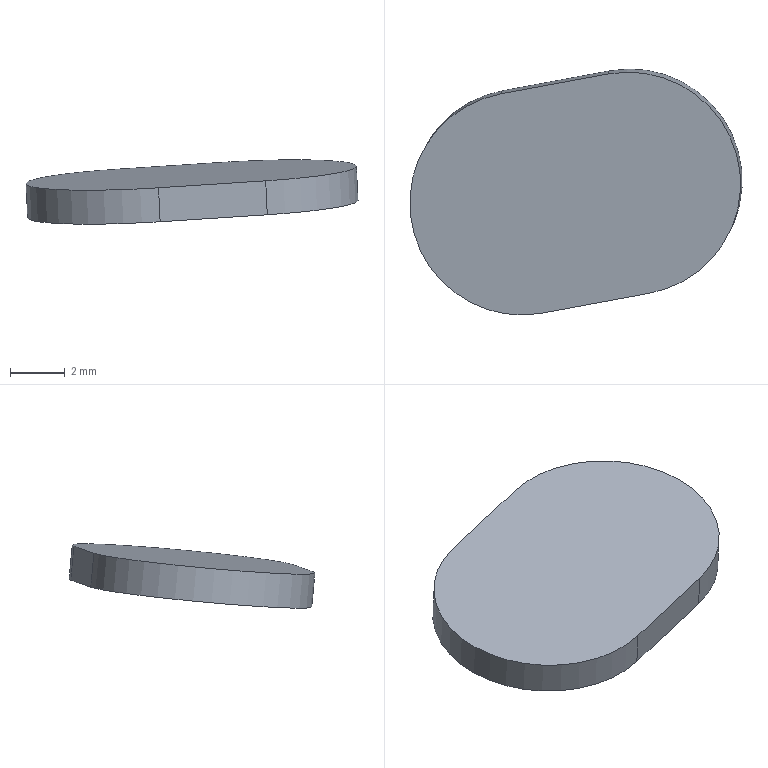Part | STEP file | gslz 2016.10.28-13_id1330_x_t | 1 solid | 6 faces | box 12.175 x 9.008 x 2.356 mm | volume 107.013 mm3 | plane 4 | cylinder 2 | commonest cylinder face diameters 8.2 x2
STEP:
#1=CARTESIAN_POINT('',(0.,0.,0.));
#2=DIRECTION('',(0.,0.,1.));
#3=DIRECTION('',(1.,0.,0.));
#4=AXIS2_PLACEMENT_3D('',#1,#2,#3);
#5=CARTESIAN_POINT('',(1413.762,14.955,-0.7524));
#6=VERTEX_POINT('',#5);
#7=CARTESIAN_POINT('',(1412.231,22.982,-0.07377));
#8=VERTEX_POINT('',#7);
#9=CARTESIAN_POINT('',(1412.996,18.968,-0.4131));
#10=DIRECTION('',(0.04745,0.09314,-0.9945));
#11=DIRECTION('',(0.4515,0.8861,0.1045));
#12=AXIS2_PLACEMENT_3D('',#9,#10,#11);
#13=CIRCLE('',#12,4.1);
#14=CARTESIAN_POINT('',(1413.056,19.085,-1.656));
#15=DIRECTION('',(-0.04745,-0.09314,0.9945));
#16=DIRECTION('',(0.,-0.9956,-0.09324));
#17=AXIS2_PLACEMENT_3D('',#14,#15,#16);
#18=CYLINDRICAL_SURFACE('',#17,4.1);
#19=CARTESIAN_POINT('',(8.956,1.25));
#20=DIRECTION('',(-1.,0.));
#21=VECTOR('',#20,1.);
#22=LINE('',#19,#21);
#23=(GEOMETRIC_REPRESENTATION_CONTEXT(2)PARAMETRIC_REPRESENTATION_CONTEXT()REPRESENTATION_CONTEXT('',''));
#24=DEFINITIONAL_REPRESENTATION('',(#22),#23);
#25=PCURVE('',#18,#24);
#26=CARTESIAN_POINT('',(1412.996,18.968,-0.4131));
#27=DIRECTION('',(0.04745,0.09314,-0.9945));
#28=DIRECTION('',(0.,0.9956,0.09324));
#29=AXIS2_PLACEMENT_3D('',#26,#27,#28);
#30=PLANE('',#29);
#31=CARTESIAN_POINT('',(0.,0.));
#32=DIRECTION('',(0.892,0.452));
#33=AXIS2_PLACEMENT_2D('',#31,#32);
#34=CIRCLE('',#33,4.1);
#35=(GEOMETRIC_REPRESENTATION_CONTEXT(2)PARAMETRIC_REPRESENTATION_CONTEXT()REPRESENTATION_CONTEXT('',''));
#36=DEFINITIONAL_REPRESENTATION('',(#34),#35);
#37=PCURVE('',#30,#36);
#38=SURFACE_CURVE('',#13,(#25,#37),.PCURVE_S1.);
#39=EDGE_CURVE('',#6,#8,#38,.T.);
#40=ORIENTED_EDGE('',*,*,#39,.T.);
#41=CARTESIAN_POINT('',(1412.29,23.098,-1.317));
#42=VERTEX_POINT('',#41);
#43=CARTESIAN_POINT('',(1412.29,23.098,-1.317));
#44=DIRECTION('',(-0.04745,-0.09314,0.9945));
#45=VECTOR('',#44,1.);
#46=LINE('',#43,#45);
#47=CARTESIAN_POINT('',(3.33,0.));
#48=DIRECTION('',(0.,1.));
#49=VECTOR('',#48,1.);
#50=LINE('',#47,#49);
#51=(GEOMETRIC_REPRESENTATION_CONTEXT(2)PARAMETRIC_REPRESENTATION_CONTEXT()REPRESENTATION_CONTEXT('',''));
#52=DEFINITIONAL_REPRESENTATION('',(#50),#51);
#53=PCURVE('',#18,#52);
#54=CARTESIAN_POINT('',(1412.29,23.098,-1.317));
#55=DIRECTION('',(0.1867,-0.9789,-0.08276));
#56=DIRECTION('',(0.9823,0.1874,0.));
#57=AXIS2_PLACEMENT_3D('',#54,#55,#56);
#58=PLANE('',#57);
#59=CARTESIAN_POINT('',(0.,0.));
#60=DIRECTION('',(-0.06407,0.9979));
#61=VECTOR('',#60,1.);
#62=LINE('',#59,#61);
#63=(GEOMETRIC_REPRESENTATION_CONTEXT(2)PARAMETRIC_REPRESENTATION_CONTEXT()REPRESENTATION_CONTEXT('',''));
#64=DEFINITIONAL_REPRESENTATION('',(#62),#63);
#65=PCURVE('',#58,#64);
#66=SURFACE_CURVE('',#46,(#53,#65),.PCURVE_S1.);
#67=EDGE_CURVE('',#42,#8,#66,.T.);
#68=ORIENTED_EDGE('',*,*,#67,.F.);
#69=CARTESIAN_POINT('',(1413.821,15.071,-1.996));
#70=VERTEX_POINT('',#69);
#71=CARTESIAN_POINT('',(1413.056,19.085,-1.656));
#72=DIRECTION('',(0.04745,0.09314,-0.9945));
#73=DIRECTION('',(0.4515,0.8861,0.1045));
#74=AXIS2_PLACEMENT_3D('',#71,#72,#73);
#75=CIRCLE('',#74,4.1);
#76=CARTESIAN_POINT('',(8.956,0.));
#77=DIRECTION('',(-1.,0.));
#78=VECTOR('',#77,1.);
#79=LINE('',#76,#78);
#80=(GEOMETRIC_REPRESENTATION_CONTEXT(2)PARAMETRIC_REPRESENTATION_CONTEXT()REPRESENTATION_CONTEXT('',''));
#81=DEFINITIONAL_REPRESENTATION('',(#79),#80);
#82=PCURVE('',#18,#81);
#83=CARTESIAN_POINT('',(1413.056,19.085,-1.656));
#84=DIRECTION('',(0.04745,0.09314,-0.9945));
#85=DIRECTION('',(0.,0.9956,0.09324));
#86=AXIS2_PLACEMENT_3D('',#83,#84,#85);
#87=PLANE('',#86);
#88=CARTESIAN_POINT('',(0.,0.));
#89=DIRECTION('',(0.892,0.452));
#90=AXIS2_PLACEMENT_2D('',#88,#89);
#91=CIRCLE('',#90,4.1);
#92=(GEOMETRIC_REPRESENTATION_CONTEXT(2)PARAMETRIC_REPRESENTATION_CONTEXT()REPRESENTATION_CONTEXT('',''));
#93=DEFINITIONAL_REPRESENTATION('',(#91),#92);
#94=PCURVE('',#87,#93);
#95=SURFACE_CURVE('',#75,(#82,#94),.PCURVE_S1.);
#96=EDGE_CURVE('',#70,#42,#95,.T.);
#97=ORIENTED_EDGE('',*,*,#96,.F.);
#98=CARTESIAN_POINT('',(1413.821,15.071,-1.996));
#99=DIRECTION('',(-0.04745,-0.09314,0.9945));
#100=VECTOR('',#99,1.);
#101=LINE('',#98,#100);
#102=CARTESIAN_POINT('',(6.471,0.));
#103=DIRECTION('',(0.,1.));
#104=VECTOR('',#103,1.);
#105=LINE('',#102,#104);
#106=(GEOMETRIC_REPRESENTATION_CONTEXT(2)PARAMETRIC_REPRESENTATION_CONTEXT()REPRESENTATION_CONTEXT('',''));
#107=DEFINITIONAL_REPRESENTATION('',(#105),#106);
#108=PCURVE('',#18,#107);
#109=CARTESIAN_POINT('',(1417.746,15.798,-1.74));
#110=DIRECTION('',(-0.1867,0.9789,0.08276));
#111=DIRECTION('',(-0.9823,-0.1874,0.));
#112=AXIS2_PLACEMENT_3D('',#109,#110,#111);
#113=PLANE('',#112);
#114=CARTESIAN_POINT('',(3.992,-0.2563));
#115=DIRECTION('',(0.06407,0.9979));
#116=VECTOR('',#115,1.);
#117=LINE('',#114,#116);
#118=(GEOMETRIC_REPRESENTATION_CONTEXT(2)PARAMETRIC_REPRESENTATION_CONTEXT()REPRESENTATION_CONTEXT('',''));
#119=DEFINITIONAL_REPRESENTATION('',(#117),#118);
#120=PCURVE('',#113,#119);
#121=SURFACE_CURVE('',#101,(#108,#120),.PCURVE_S1.);
#122=EDGE_CURVE('',#70,#6,#121,.T.);
#123=ORIENTED_EDGE('',*,*,#122,.T.);
#124=EDGE_LOOP('',(#40,#68,#97,#123));
#125=FACE_BOUND('',#124,.T.);
#126=ADVANCED_FACE('',(#125),#18,.T.);
#127=CARTESIAN_POINT('',(1416.156,23.709,0.1816));
#128=VERTEX_POINT('',#127);
#129=CARTESIAN_POINT('',(1412.231,22.982,-0.07377));
#130=DIRECTION('',(0.9813,0.1818,0.06385));
#131=VECTOR('',#130,1.);
#132=LINE('',#129,#131);
#133=CARTESIAN_POINT('',(-0.08008,1.247));
#134=DIRECTION('',(0.9979,0.06407));
#135=VECTOR('',#134,1.);
#136=LINE('',#133,#135);
#137=(GEOMETRIC_REPRESENTATION_CONTEXT(2)PARAMETRIC_REPRESENTATION_CONTEXT()REPRESENTATION_CONTEXT('',''));
#138=DEFINITIONAL_REPRESENTATION('',(#136),#137);
#139=PCURVE('',#58,#138);
#140=CARTESIAN_POINT('',(4.028,-0.7665));
#141=DIRECTION('',(0.1869,0.9824));
#142=VECTOR('',#141,1.);
#143=LINE('',#140,#142);
#144=(GEOMETRIC_REPRESENTATION_CONTEXT(2)PARAMETRIC_REPRESENTATION_CONTEXT()REPRESENTATION_CONTEXT('',''));
#145=DEFINITIONAL_REPRESENTATION('',(#143),#144);
#146=PCURVE('',#30,#145);
#147=SURFACE_CURVE('',#132,(#139,#146),.PCURVE_S1.);
#148=EDGE_CURVE('',#8,#128,#147,.T.);
#149=ORIENTED_EDGE('',*,*,#148,.T.);
#150=CARTESIAN_POINT('',(1416.215,23.826,-1.062));
#151=VERTEX_POINT('',#150);
#152=CARTESIAN_POINT('',(1416.215,23.826,-1.062));
#153=DIRECTION('',(-0.04745,-0.09314,0.9945));
#154=VECTOR('',#153,1.);
#155=LINE('',#152,#154);
#156=CARTESIAN_POINT('',(3.992,0.2563));
#157=DIRECTION('',(-0.06407,0.9979));
#158=VECTOR('',#157,1.);
#159=LINE('',#156,#158);
#160=(GEOMETRIC_REPRESENTATION_CONTEXT(2)PARAMETRIC_REPRESENTATION_CONTEXT()REPRESENTATION_CONTEXT('',''));
#161=DEFINITIONAL_REPRESENTATION('',(#159),#160);
#162=PCURVE('',#58,#161);
#163=CARTESIAN_POINT('',(1416.981,19.812,-1.401));
#164=DIRECTION('',(-0.04745,-0.09314,0.9945));
#165=DIRECTION('',(0.,-0.9956,-0.09324));
#166=AXIS2_PLACEMENT_3D('',#163,#164,#165);
#167=CYLINDRICAL_SURFACE('',#166,4.1);
#168=CARTESIAN_POINT('',(3.33,0.));
#169=DIRECTION('',(0.,1.));
#170=VECTOR('',#169,1.);
#171=LINE('',#168,#170);
#172=(GEOMETRIC_REPRESENTATION_CONTEXT(2)PARAMETRIC_REPRESENTATION_CONTEXT()REPRESENTATION_CONTEXT('',''));
#173=DEFINITIONAL_REPRESENTATION('',(#171),#172);
#174=PCURVE('',#167,#173);
#175=SURFACE_CURVE('',#155,(#162,#174),.PCURVE_S1.);
#176=EDGE_CURVE('',#151,#128,#175,.T.);
#177=ORIENTED_EDGE('',*,*,#176,.F.);
#178=CARTESIAN_POINT('',(1412.29,23.098,-1.317));
#179=DIRECTION('',(0.9813,0.1818,0.06385));
#180=VECTOR('',#179,1.);
#181=LINE('',#178,#180);
#182=CARTESIAN_POINT('',(0.,0.));
#183=DIRECTION('',(0.9979,0.06407));
#184=VECTOR('',#183,1.);
#185=LINE('',#182,#184);
#186=(GEOMETRIC_REPRESENTATION_CONTEXT(2)PARAMETRIC_REPRESENTATION_CONTEXT()REPRESENTATION_CONTEXT('',''));
#187=DEFINITIONAL_REPRESENTATION('',(#185),#186);
#188=PCURVE('',#58,#187);
#189=CARTESIAN_POINT('',(4.028,-0.7665));
#190=DIRECTION('',(0.1869,0.9824));
#191=VECTOR('',#190,1.);
#192=LINE('',#189,#191);
#193=(GEOMETRIC_REPRESENTATION_CONTEXT(2)PARAMETRIC_REPRESENTATION_CONTEXT()REPRESENTATION_CONTEXT('',''));
#194=DEFINITIONAL_REPRESENTATION('',(#192),#193);
#195=PCURVE('',#87,#194);
#196=SURFACE_CURVE('',#181,(#188,#195),.PCURVE_S1.);
#197=EDGE_CURVE('',#42,#151,#196,.T.);
#198=ORIENTED_EDGE('',*,*,#197,.F.);
#199=ORIENTED_EDGE('',*,*,#67,.T.);
#200=EDGE_LOOP('',(#149,#177,#198,#199));
#201=FACE_BOUND('',#200,.T.);
#202=ADVANCED_FACE('',(#201),#58,.F.);
#203=CARTESIAN_POINT('',(1417.687,15.682,-0.497));
#204=VERTEX_POINT('',#203);
#205=CARTESIAN_POINT('',(1416.921,19.696,-0.1577));
#206=DIRECTION('',(0.04745,0.09314,-0.9945));
#207=DIRECTION('',(0.4515,0.8861,0.1045));
#208=AXIS2_PLACEMENT_3D('',#205,#206,#207);
#209=CIRCLE('',#208,4.1);
#210=CARTESIAN_POINT('',(8.956,1.25));
#211=DIRECTION('',(-1.,0.));
#212=VECTOR('',#211,1.);
#213=LINE('',#210,#212);
#214=(GEOMETRIC_REPRESENTATION_CONTEXT(2)PARAMETRIC_REPRESENTATION_CONTEXT()REPRESENTATION_CONTEXT('',''));
#215=DEFINITIONAL_REPRESENTATION('',(#213),#214);
#216=PCURVE('',#167,#215);
#217=CARTESIAN_POINT('',(0.7478,3.929));
#218=DIRECTION('',(0.892,0.452));
#219=AXIS2_PLACEMENT_2D('',#217,#218);
#220=CIRCLE('',#219,4.1);
#221=(GEOMETRIC_REPRESENTATION_CONTEXT(2)PARAMETRIC_REPRESENTATION_CONTEXT()REPRESENTATION_CONTEXT('',''));
#222=DEFINITIONAL_REPRESENTATION('',(#220),#221);
#223=PCURVE('',#30,#222);
#224=SURFACE_CURVE('',#209,(#216,#223),.PCURVE_S1.);
#225=EDGE_CURVE('',#128,#204,#224,.T.);
#226=ORIENTED_EDGE('',*,*,#225,.T.);
#227=CARTESIAN_POINT('',(1417.746,15.798,-1.74));
#228=VERTEX_POINT('',#227);
#229=CARTESIAN_POINT('',(1417.746,15.798,-1.74));
#230=DIRECTION('',(-0.04745,-0.09314,0.9945));
#231=VECTOR('',#230,1.);
#232=LINE('',#229,#231);
#233=CARTESIAN_POINT('',(0.1881,0.));
#234=DIRECTION('',(0.,1.));
#235=VECTOR('',#234,1.);
#236=LINE('',#233,#235);
#237=(GEOMETRIC_REPRESENTATION_CONTEXT(2)PARAMETRIC_REPRESENTATION_CONTEXT()REPRESENTATION_CONTEXT('',''));
#238=DEFINITIONAL_REPRESENTATION('',(#236),#237);
#239=PCURVE('',#167,#238);
#240=CARTESIAN_POINT('',(0.,0.));
#241=DIRECTION('',(0.06407,0.9979));
#242=VECTOR('',#241,1.);
#243=LINE('',#240,#242);
#244=(GEOMETRIC_REPRESENTATION_CONTEXT(2)PARAMETRIC_REPRESENTATION_CONTEXT()REPRESENTATION_CONTEXT('',''));
#245=DEFINITIONAL_REPRESENTATION('',(#243),#244);
#246=PCURVE('',#113,#245);
#247=SURFACE_CURVE('',#232,(#239,#246),.PCURVE_S1.);
#248=EDGE_CURVE('',#228,#204,#247,.T.);
#249=ORIENTED_EDGE('',*,*,#248,.F.);
#250=CARTESIAN_POINT('',(1416.981,19.812,-1.401));
#251=DIRECTION('',(0.04745,0.09314,-0.9945));
#252=DIRECTION('',(0.4515,0.8861,0.1045));
#253=AXIS2_PLACEMENT_3D('',#250,#251,#252);
#254=CIRCLE('',#253,4.1);
#255=CARTESIAN_POINT('',(8.956,0.));
#256=DIRECTION('',(-1.,0.));
#257=VECTOR('',#256,1.);
#258=LINE('',#255,#257);
#259=(GEOMETRIC_REPRESENTATION_CONTEXT(2)PARAMETRIC_REPRESENTATION_CONTEXT()REPRESENTATION_CONTEXT('',''));
#260=DEFINITIONAL_REPRESENTATION('',(#258),#259);
#261=PCURVE('',#167,#260);
#262=CARTESIAN_POINT('',(0.7478,3.929));
#263=DIRECTION('',(0.892,0.452));
#264=AXIS2_PLACEMENT_2D('',#262,#263);
#265=CIRCLE('',#264,4.1);
#266=(GEOMETRIC_REPRESENTATION_CONTEXT(2)PARAMETRIC_REPRESENTATION_CONTEXT()REPRESENTATION_CONTEXT('',''));
#267=DEFINITIONAL_REPRESENTATION('',(#265),#266);
#268=PCURVE('',#87,#267);
#269=SURFACE_CURVE('',#254,(#261,#268),.PCURVE_S1.);
#270=EDGE_CURVE('',#151,#228,#269,.T.);
#271=ORIENTED_EDGE('',*,*,#270,.F.);
#272=ORIENTED_EDGE('',*,*,#176,.T.);
#273=EDGE_LOOP('',(#226,#249,#271,#272));
#274=FACE_BOUND('',#273,.T.);
#275=ADVANCED_FACE('',(#274),#167,.T.);
#276=CARTESIAN_POINT('',(1417.687,15.682,-0.497));
#277=DIRECTION('',(-0.9813,-0.1818,-0.06385));
#278=VECTOR('',#277,1.);
#279=LINE('',#276,#278);
#280=CARTESIAN_POINT('',(0.08008,1.247));
#281=DIRECTION('',(0.9979,-0.06407));
#282=VECTOR('',#281,1.);
#283=LINE('',#280,#282);
#284=(GEOMETRIC_REPRESENTATION_CONTEXT(2)PARAMETRIC_REPRESENTATION_CONTEXT()REPRESENTATION_CONTEXT('',''));
#285=DEFINITIONAL_REPRESENTATION('',(#283),#284);
#286=PCURVE('',#113,#285);
#287=CARTESIAN_POINT('',(-3.28,4.696));
#288=DIRECTION('',(-0.1869,-0.9824));
#289=VECTOR('',#288,1.);
#290=LINE('',#287,#289);
#291=(GEOMETRIC_REPRESENTATION_CONTEXT(2)PARAMETRIC_REPRESENTATION_CONTEXT()REPRESENTATION_CONTEXT('',''));
#292=DEFINITIONAL_REPRESENTATION('',(#290),#291);
#293=PCURVE('',#30,#292);
#294=SURFACE_CURVE('',#279,(#286,#293),.PCURVE_S1.);
#295=EDGE_CURVE('',#204,#6,#294,.T.);
#296=ORIENTED_EDGE('',*,*,#295,.T.);
#297=ORIENTED_EDGE('',*,*,#122,.F.);
#298=CARTESIAN_POINT('',(1417.746,15.798,-1.74));
#299=DIRECTION('',(-0.9813,-0.1818,-0.06385));
#300=VECTOR('',#299,1.);
#301=LINE('',#298,#300);
#302=CARTESIAN_POINT('',(0.,0.));
#303=DIRECTION('',(0.9979,-0.06407));
#304=VECTOR('',#303,1.);
#305=LINE('',#302,#304);
#306=(GEOMETRIC_REPRESENTATION_CONTEXT(2)PARAMETRIC_REPRESENTATION_CONTEXT()REPRESENTATION_CONTEXT('',''));
#307=DEFINITIONAL_REPRESENTATION('',(#305),#306);
#308=PCURVE('',#113,#307);
#309=CARTESIAN_POINT('',(-3.28,4.696));
#310=DIRECTION('',(-0.1869,-0.9824));
#311=VECTOR('',#310,1.);
#312=LINE('',#309,#311);
#313=(GEOMETRIC_REPRESENTATION_CONTEXT(2)PARAMETRIC_REPRESENTATION_CONTEXT()REPRESENTATION_CONTEXT('',''));
#314=DEFINITIONAL_REPRESENTATION('',(#312),#313);
#315=PCURVE('',#87,#314);
#316=SURFACE_CURVE('',#301,(#308,#315),.PCURVE_S1.);
#317=EDGE_CURVE('',#228,#70,#316,.T.);
#318=ORIENTED_EDGE('',*,*,#317,.F.);
#319=ORIENTED_EDGE('',*,*,#248,.T.);
#320=EDGE_LOOP('',(#296,#297,#318,#319));
#321=FACE_BOUND('',#320,.T.);
#322=ADVANCED_FACE('',(#321),#113,.F.);
#323=ORIENTED_EDGE('',*,*,#96,.T.);
#324=ORIENTED_EDGE('',*,*,#197,.T.);
#325=ORIENTED_EDGE('',*,*,#270,.T.);
#326=ORIENTED_EDGE('',*,*,#317,.T.);
#327=EDGE_LOOP('',(#323,#324,#325,#326));
#328=FACE_BOUND('',#327,.T.);
#329=ADVANCED_FACE('',(#328),#87,.T.);
#330=ORIENTED_EDGE('',*,*,#39,.F.);
#331=ORIENTED_EDGE('',*,*,#295,.F.);
#332=ORIENTED_EDGE('',*,*,#225,.F.);
#333=ORIENTED_EDGE('',*,*,#148,.F.);
#334=EDGE_LOOP('',(#330,#331,#332,#333));
#335=FACE_BOUND('',#334,.T.);
#336=ADVANCED_FACE('',(#335),#30,.F.);
#337=CLOSED_SHELL('',(#126,#202,#275,#322,#329,#336));
#338=MANIFOLD_SOLID_BREP('',#337);
#339=(LENGTH_UNIT()NAMED_UNIT(*)SI_UNIT(.MILLI.,.METRE.));
#340=UNCERTAINTY_MEASURE_WITH_UNIT(LENGTH_MEASURE(0.0000001),#339,'','');
#341=(NAMED_UNIT(*)PLANE_ANGLE_UNIT()SI_UNIT($,.RADIAN.));
#342=(NAMED_UNIT(*)SI_UNIT($,.STERADIAN.)SOLID_ANGLE_UNIT());
#343=(GEOMETRIC_REPRESENTATION_CONTEXT(3)GLOBAL_UNCERTAINTY_ASSIGNED_CONTEXT((#340))GLOBAL_UNIT_ASSIGNED_CONTEXT((#339,#341,#342))REPRESENTATION_CONTEXT('',''));
#344=ADVANCED_BREP_SHAPE_REPRESENTATION('',(#4,#338),#343);